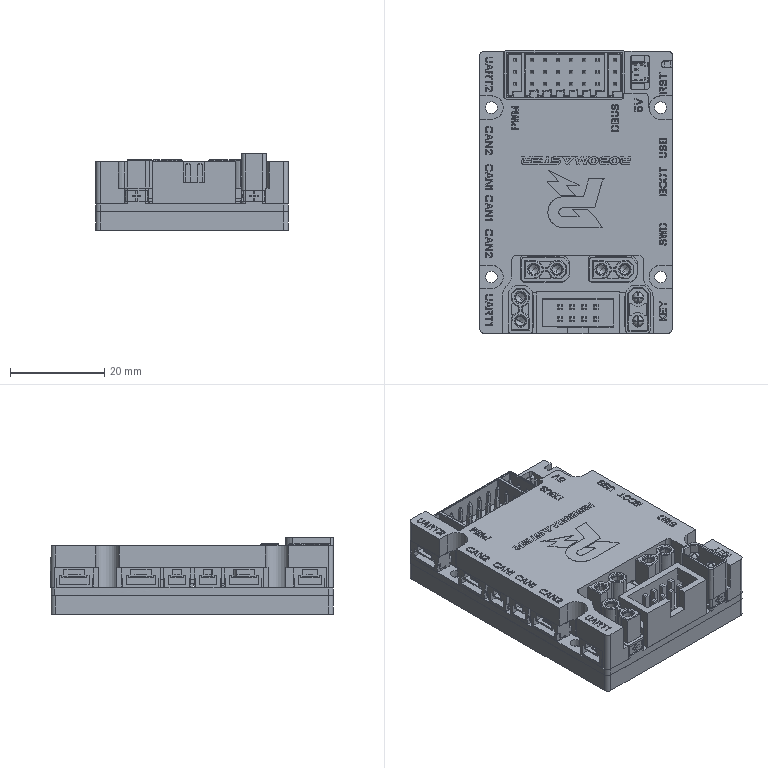Part | SolidWorks | features BaseBody 8 | 8 solids | 6286 faces | volume 22684 mm3 | plane 4797 | cylinder 1015 | sphere 205 | spline 179 | cone 90 | commonest cylinder face diameters 1 x98 2 x60 0.4 x59 0.6 x59 0.2 x58 0.8 x56